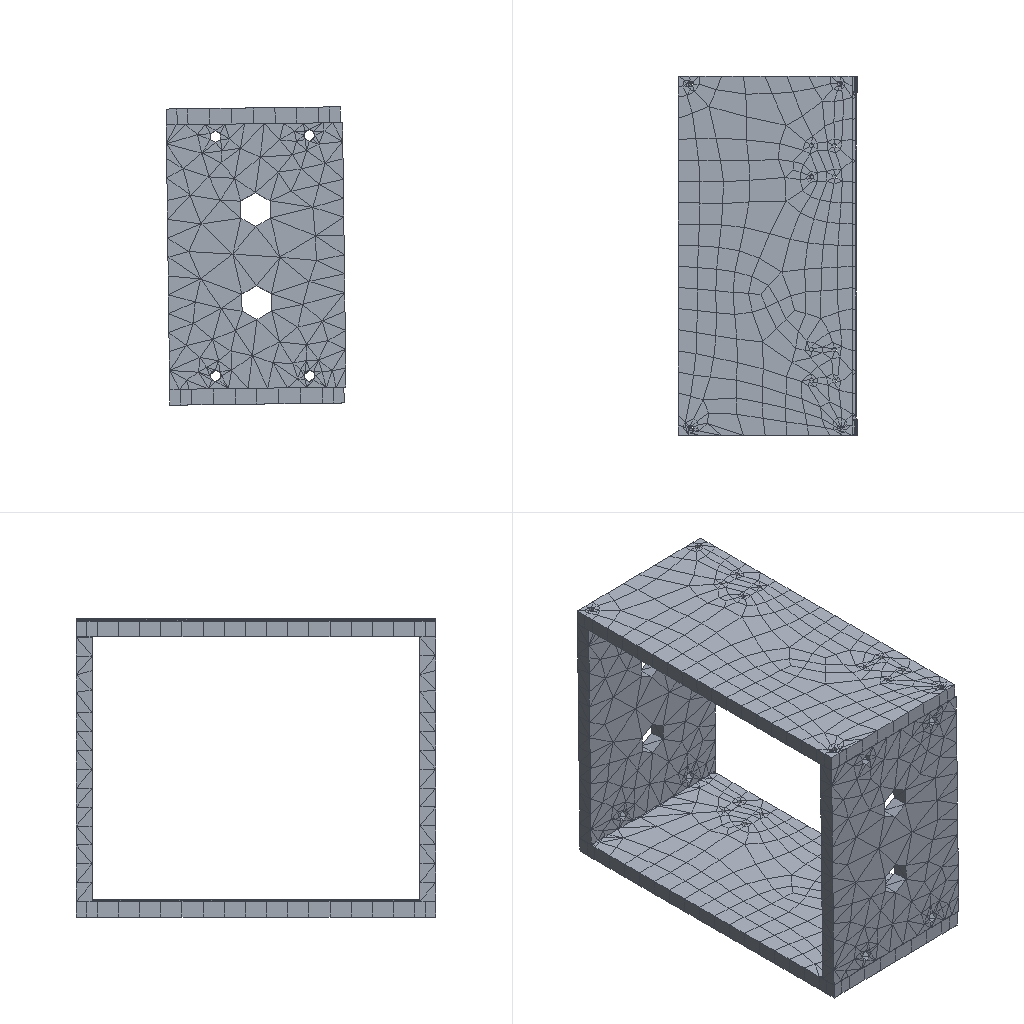Simulation study | ansys workbench
Ansys APDL input file, long lists of numbers shortened:
/batch
/config,noeldb,1     ! force off writing results to database
*get,_wallstrt,active,,time,wall
! ANSYS input file written by Workbench version 2022 R1
! File used for geometry attach: F:\ansys（分析文件汇总)\破碎机有限元分析\机架.STEP
/title,wbnew--____ (B5)
! ****** Begin Custom Load Command Snippet ******
/COM, ACT Extensions:
/COM,     LSDYNA, 2021.1
/COM,
! ****** End   Custom Load Command Snippet ******
*DIM,_wb_ProjectScratch_dir,string,248
_wb_ProjectScratch_dir(1) = 'C:\Users\Administrator\AppData\Local\Temp\WB_Administrator_9184_2\_ProjectScratch\ScrCD6D\'
*DIM,_wb_SolverFiles_dir,string,248
_wb_SolverFiles_dir(1) = 'C:\Users\Administrator\AppData\Local\Temp\WB_Administrator_9184_2\wbnew_files\dp0\SYS\MECH\'
*DIM,_wb_userfiles_dir,string,248
_wb_userfiles_dir(1) = 'C:\Users\Administrator\AppData\Local\Temp\WB_Administrator_9184_2\wbnew_files\user_files\'
/com,--- Data in consistent NMM units. See Solving Units in the help system for more information.
/units,MPA
/nopr
/wb,file,start              !  signify a WB generated input file
/prep7
! Turn off shape checking because checks already performed inside WB mesher.
! See help system for more information.
SHPP,OFF,,NOWARN
/nolist
etcon,set             ! allow ANSYS to choose best KEYOP's for 180x elements, resets any applicable keyopt to MAPDL defaults
/com,*********** Nodes for the whole assembly ***********
nblock,3,,29249
(1i9,3e20.9e3)
        1    -2.575000754E+02     5.592090867E+02    -2.535723079E+02
! (26589 more lines like these left out)
-1
/wb,elem,start            !  set before creation of elements
/com,*********** Elements for Body 1 "__-FreeParts|Mirror3" ***********
et,1,186
keyo,1,2,1          ! set full integration on SOLID186
eblock,19,solid,,31
(19i9)
        1        1        1        1        0        0        0        0       20        0       26      237      248      252      243      268      257      253      262
! (61 more lines like these left out)
-1
/com,*********** Elements for Body 2 "__-FreeParts|Gusset1" ***********
et,2,186
keyo,2,2,1          ! set full integration on SOLID186
eblock,19,solid,,25
(19i9)
        2        2        2        2        0        0        0        0       20        0        1        1        2        7        9       26       25       20       18
! (49 more lines like these left out)
-1
/com,*********** Elements for Body 3 "__-FreeParts|Fillet12" ***********
et,3,187
eblock,19,solid,,13867
(19i9)
        3        3        3        3        0        0        0        0       10        0       57     1498     4616     3445     4609    11767    22290    11762    11766
! (27733 more lines like these left out)
-1
/wb,elem,end               !  done creating elements
/com,*********** Send User Defined Coordinate System(s) ***********
csys,0
toffst,273.15,  ! Temperature offset from absolute zero
/com,*********** Set Reference Temperature ***********
tref,22.
/wb,mat,start              !  starting to send materials
/com,*********** Send Materials ***********
Temperature = 'TEMP' ! Temperature
MP,DENS,1,7.85e-09,	! tonne mm^-3
MP,ALPX,1,1.2e-05,	! C^-1
MP,C,1,434000000,	! mm^2 s^-2 C^-1
MP,KXX,1,60.5,	! tonne mm s^-3 C^-1
MP,RSVX,1,0.00017,	! ohm mm
MP,EX,1,200000,	! tonne s^-2 mm^-1
MP,NUXY,1,0.3,
MP,MURX,1,10000,
Temperature = 'TEMP' ! Temperature
MP,DENS,2,7.85e-09,	! tonne mm^-3
MP,ALPX,2,1.2e-05,	! C^-1
MP,C,2,434000000,	! mm^2 s^-2 C^-1
MP,KXX,2,60.5,	! tonne mm s^-3 C^-1
MP,RSVX,2,0.00017,	! ohm mm
MP,EX,2,200000,	! tonne s^-2 mm^-1
MP,NUXY,2,0.3,
MP,MURX,2,10000,
Temperature = 'TEMP' ! Temperature
MP,DENS,3,7.85e-09,	! tonne mm^-3
MP,ALPX,3,1.2e-05,	! C^-1
MP,C,3,434000000,	! mm^2 s^-2 C^-1
MP,KXX,3,60.5,	! tonne mm s^-3 C^-1
MP,RSVX,3,0.00017,	! ohm mm
MP,EX,3,200000,	! tonne s^-2 mm^-1
MP,NUXY,3,0.3,
MP,MURX,3,10000,
/wb,mat,end                !  done sending materials
!************************* Model Summary ********************
!__-FreeParts|Mirror3,	结构钢,	matid,	1
!__-FreeParts|Gusset1,	结构钢,	matid,	2
!__-FreeParts|Fillet12,	结构钢,	matid,	3
!************************* End Model Summary ********************
! get the diagonal of the bounding box. Needed later for other things
*get,_xmin,node,,mnloc,x
*get,_ymin,node,,mnloc,y
*get,_zmin,node,,mnloc,z
*get,_xmax,node,,mxloc,x
*get,_ymax,node,,mxloc,y
*get,_zmax,node,,mxloc,z
_ASMDIAG=(_xmax-_xmin)*(_xmax-_xmin)+(_ymax-_ymin)*(_ymax-_ymin)+(_zmax-_zmin)*(_zmax-_zmin)
_ASMDIAG=SQRT(_ASMDIAG)
/wb,contact,start          !  starting to send contact
/com,*********** Create Contact "接触区域" ***********
/com,            Real Constant Set For Above Contact Is 5 & 4
*set,tid,5
*set,cid,4
r,tid
r,cid
et,tid,170
et,cid,174
eblock,10,,,14
(15i9)
    21024        5        5        5        0      294      296      302      295      482      485      483      481
! (13 more lines like these left out)
-1
eblock,10,,,14
(15i9)
    21038        4        4        4        0      294      296      302      295      482      485      483      481
! (13 more lines like these left out)
-1
eblock,10,,,43
(15i9)
    21052        4        5        4        0      876     2351      886      886     7467     7545      886     7466
! (42 more lines like these left out)
-1
eblock,10,,,43
(15i9)
    21095        5        4        5        0      876     2351      886      886     7467     7545      886     7466
! (42 more lines like these left out)
-1
keyo,cid,8,2               ! auto create asymmetric contact (from Program Controlled setting)
keyo,cid,10,0              ! adjust contact stiffness each NR iteration (from Program Controlled setting)
keyo,cid,12,5              ! bonded always
keyo,cid,18,1              ! small sliding turned on by application
keyo,cid,2,0               ! augmented Lagrange (from Program Controlled setting)
keyo,cid,4,0               ! on Gauss point (from Program Controlled setting)
keyo,cid,9,1               ! ignore initial gaps/penetration
keyo,cid,7,0               ! No Prediction
rmod,tid,3,10.      ! FKN
rmod,tid,5,0.       ! ICONT
rmod,tid,6,0.       ! PINB
rmod,tid,10,0.      ! CNOF
rmod,tid,12,0.      ! FKT
rmod,tid,36,32      ! WB DSID
rmod,cid,3,10.      ! FKN
rmod,cid,5,0.       ! ICONT
rmod,cid,6,0.       ! PINB
rmod,cid,10,0.      ! CNOF
rmod,cid,12,0.      ! FKT
rmod,cid,36,32      ! WB DSID
/com,*********** Create Contact "接触区域 2" ***********
/com,            Real Constant Set For Above Contact Is 7 & 6
*set,tid,7
*set,cid,6
r,tid
r,cid
et,tid,170
et,cid,174
eblock,10,,,14
(15i9)
    21138        7        7        7        0       44       56       57       43      196      214      194      193
! (13 more lines like these left out)
-1
eblock,10,,,14
(15i9)
    21152        6        6        6        0       44       56       57       43      196      214      194      193
! (13 more lines like these left out)
-1
eblock,10,,,36
(15i9)
    21166        6        7        6        0      872     2002     4860     4860     7428    15365     4860     7438
! (35 more lines like these left out)
-1
eblock,10,,,36
(15i9)
    21202        7        6        7        0      872     2002     4860     4860     7428    15365     4860     7438
! (35 more lines like these left out)
-1
keyo,cid,8,2               ! auto create asymmetric contact (from Program Controlled setting)
keyo,cid,10,0              ! adjust contact stiffness each NR iteration (from Program Controlled setting)
keyo,cid,12,5              ! bonded always
keyo,cid,18,1              ! small sliding turned on by application
keyo,cid,2,0               ! augmented Lagrange (from Program Controlled setting)
keyo,cid,4,0               ! on Gauss point (from Program Controlled setting)
keyo,cid,9,1               ! ignore initial gaps/penetration
keyo,cid,7,0               ! No Prediction
rmod,tid,3,10.      ! FKN
rmod,tid,5,0.       ! ICONT
rmod,tid,6,0.       ! PINB
rmod,tid,10,0.      ! CNOF
rmod,tid,12,0.      ! FKT
rmod,tid,36,35      ! WB DSID
rmod,cid,3,10.      ! FKN
rmod,cid,5,0.       ! ICONT
rmod,cid,6,0.       ! PINB
rmod,cid,10,0.      ! CNOF
rmod,cid,12,0.      ! FKT
rmod,cid,36,35      ! WB DSID
nsel,all
esel,all
/wb,contact,end            !  done creating contacts
/golist
/wb,load,start             !  starting to send loads
/com,*********** Fixed Supports ***********
CMBLOCK,_FIXEDSU,NODE,      668
(8i10)
         1         2         3         4         5         6         7         8
! (83 more lines like these left out)
cmsel,s,_FIXEDSU
d,all,all
nsel,all
/com,*********** Define Force Using Surface Effect Elements ***********
local,12,0,0.,0.,0.,0.,0.,0.
csys,0
et,8,154
eblock,10,,,223
(15i9)
    21238        8        8        8       12     1288     1300     2658     2658    10257    10315     2658    10260
! (222 more lines like these left out)
-1
esel,s,type,,8
keyop,8,2,1                ! Apply load in local coordinate system
keyop,8,7,1                ! Use original area so load is constant in large deformation
esel,all
/gst,on,on
fini
*get,_numnode,node,0,count
*get,_numelem,elem,0,count
*get, _MAXELEMNUM, elem, 0, NUM, MAX
*get, _MAXNODENUM, node, 0, NUM, MAX
*get, _MAXELEMTYPE, etyp, 0, NUM, MAX
*get, _MAXREALCONST, real, 0, NUM, MAX
/go
/wb,load,end               !  done creating loads
/com,--- Number of total nodes = %_numnode%
/com,--- Number of contact elements = 437
/com,--- Number of spring elements = 0
/com,--- Number of bearing elements = 0
/com,--- Number of solid elements = 13923
/com,--- Number of condensed parts = 0
/com,--- Number of total elements = %_numelem%
*get,_wallbsol,active,,time,wall
/com,****************************************************************************
/com,*************************    SOLUTION       ********************************
/com,****************************************************************************
/solu
antype,0                   ! static analysis
_thickRatio=0.333   ! Ratio of thick parts in the model
eqsl,sparse,,,,,1
cntr,print,1               ! print out contact info and also make no initial contact an error
dmpoption,emat,no             ! Don't combine emat file for DANSYS
dmpoption,esav,no             ! Don't combine esav file for DANSYS
nldiag,cont,iter           ! print out contact info each equilibrium iteration
rescontrol,,none                 ! Do not keep any restart files
/com,****************************************************
/com,******************* SOLVE FOR LS 1 OF 1 ****************
esel,s,type,,8
nsle
sfe,all,1,pres,1,0.
sfe,all,2,pres,1,2.45197536831665e-013
sfe,all,3,pres,1,0.2146
nsel,all
esel,all
/nopr
/gopr
nsub,1,1,1
time,1.
outres,erase
outres,all,none
outres,nsol,all,
outres,rsol,all
outres,eangl,all
outres,etmp,all
outres,veng,all
outres,strs,all,
outres,epel,all,
outres,eppl,all,
outres,cont,all,
! *********** WB SOLVE COMMAND ***********
! check interactive state
*get,ANSINTER_,active,,int
*if,ANSINTER_,ne,0,then
/eof
*endif
solve
/com *************** Write FE CONNECTORS *********
CEWRITE,file,ce,,INTE
/com,****************************************************
/com,*************** FINISHED SOLVE FOR LS 1 *************
*get,_wallasol,active,,time,wall
/nopr
*get,_numnode,node,0,count
*get,_numelem,elem,0,count
*get, _MAXELEMNUM, elem, 0, NUM, MAX
*get, _MAXNODENUM, node, 0, NUM, MAX,,,INTERNAL
*get, _MAXELEMTYPE, etyp, 0, NUM, MAX
*get, _MAXREALCONST, real, 0, NUM, MAX
/gopr
/post1
xmlo,ENCODING,ISO-8859-1
xmlo,parm
/xml,parm,xml
fini
/gopr
*get,_walldone,active,,time,wall
_preptime=(_wallbsol-_wallstrt)*3600
_solvtime=(_wallasol-_wallbsol)*3600
_posttime=(_walldone-_wallasol)*3600
_totaltim=(_walldone-_wallstrt)*3600
*get,_dlbratio,active,0,solu,dlbr
*get,_combtime,active,0,solu,comb
*get,_ssmode,active,0,solu,ssmm
*get,_ndofs,active,0,solu,ndof
*get,_sol_end_time,active,0,set,time
*if,_sol_end_time,eq,1.,then
/fclean				!clean distributed files
*endif
/com,--- Total number of nodes = %_numnode%
/com,--- Total number of elements = %_numelem%
/com,--- Element load balance ratio = %_dlbratio%
/com,--- Time to combine distributed files = %_combtime%
/com,--- Sparse memory mode = %_ssmode%
/com,--- Number of DOF = %_ndofs%
/wb,file,end               ! done with WB generated input